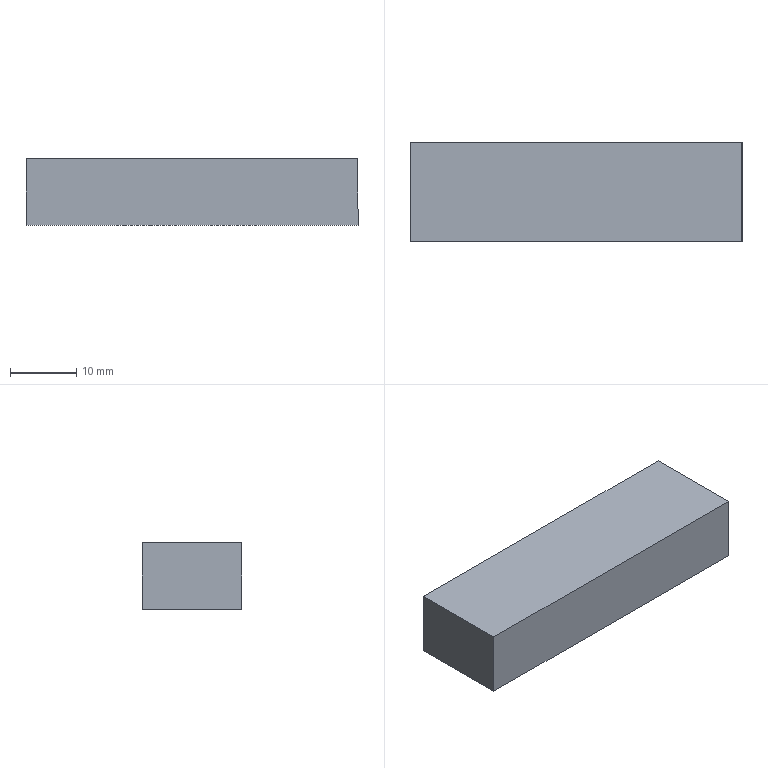Part | 4 solids | 50 faces | box 50 x 15 x 10 mm | volume 12752 mm3 | plane 42 | cylinder 8 | commonest cylinder face diameters 2.5 x4 3 x4
STEP:
#1=CARTESIAN_POINT('',(6.,12.,-2.5));
#2=VERTEX_POINT('',#1);
#3=CARTESIAN_POINT('',(6.,12.,7.5));
#4=VERTEX_POINT('',#3);
#5=CARTESIAN_POINT('',(6.,12.,2.5));
#6=DIRECTION('',(0.,0.,1.));
#7=VECTOR('',#6,1000.);
#8=LINE('',#5,#7);
#9=EDGE_CURVE('',#2,#4,#8,.T.);
#10=ORIENTED_EDGE('',*,*,#9,.F.);
#11=CARTESIAN_POINT('',(-44.,12.,-2.5));
#12=VERTEX_POINT('',#11);
#13=CARTESIAN_POINT('',(-19.,12.,-2.5));
#14=DIRECTION('',(1.,0.,0.));
#15=VECTOR('',#14,1000.);
#16=LINE('',#13,#15);
#17=EDGE_CURVE('',#12,#2,#16,.T.);
#18=ORIENTED_EDGE('',*,*,#17,.F.);
#19=CARTESIAN_POINT('',(-44.,12.,7.5));
#20=VERTEX_POINT('',#19);
#21=CARTESIAN_POINT('',(-44.,12.,2.5));
#22=DIRECTION('',(0.,0.,-1.));
#23=VECTOR('',#22,1000.);
#24=LINE('',#21,#23);
#25=EDGE_CURVE('',#20,#12,#24,.T.);
#26=ORIENTED_EDGE('',*,*,#25,.F.);
#27=CARTESIAN_POINT('',(-19.,12.,7.5));
#28=DIRECTION('',(-1.,0.,0.));
#29=VECTOR('',#28,1000.);
#30=LINE('',#27,#29);
#31=EDGE_CURVE('',#4,#20,#30,.T.);
#32=ORIENTED_EDGE('',*,*,#31,.F.);
#33=EDGE_LOOP('',(#10,#18,#26,#32));
#34=FACE_BOUND('',#33,.T.);
#35=CARTESIAN_POINT('',(-19.,12.,2.5));
#36=DIRECTION('',(0.,1.,0.));
#37=DIRECTION('',(0.,0.,1.));
#38=AXIS2_PLACEMENT_3D('',#35,#36,#37);
#39=PLANE('',#38);
#40=ADVANCED_FACE('',(#34),#39,.T.);
#41=CARTESIAN_POINT('',(6.,-3.,-2.5));
#42=VERTEX_POINT('',#41);
#43=CARTESIAN_POINT('',(6.,-3.,-2.5));
#44=DIRECTION('',(0.,1.,0.));
#45=VECTOR('',#44,1000.);
#46=LINE('',#43,#45);
#47=EDGE_CURVE('',#42,#2,#46,.T.);
#48=ORIENTED_EDGE('',*,*,#47,.T.);
#49=ORIENTED_EDGE('',*,*,#9,.T.);
#50=CARTESIAN_POINT('',(6.,-3.,7.5));
#51=VERTEX_POINT('',#50);
#52=CARTESIAN_POINT('',(6.,-3.,7.5));
#53=DIRECTION('',(0.,1.,0.));
#54=VECTOR('',#53,1000.);
#55=LINE('',#52,#54);
#56=EDGE_CURVE('',#51,#4,#55,.T.);
#57=ORIENTED_EDGE('',*,*,#56,.F.);
#58=CARTESIAN_POINT('',(6.,-3.,2.5));
#59=DIRECTION('',(0.,0.,-1.));
#60=VECTOR('',#59,1000.);
#61=LINE('',#58,#60);
#62=EDGE_CURVE('',#51,#42,#61,.T.);
#63=ORIENTED_EDGE('',*,*,#62,.T.);
#64=EDGE_LOOP('',(#48,#49,#57,#63));
#65=FACE_BOUND('',#64,.T.);
#66=CARTESIAN_POINT('',(6.,-3.,2.5));
#67=DIRECTION('',(1.,0.,0.));
#68=DIRECTION('',(0.,0.,-1.));
#69=AXIS2_PLACEMENT_3D('',#66,#67,#68);
#70=PLANE('',#69);
#71=ADVANCED_FACE('',(#65),#70,.T.);
#72=ORIENTED_EDGE('',*,*,#56,.T.);
#73=ORIENTED_EDGE('',*,*,#31,.T.);
#74=CARTESIAN_POINT('',(-44.,-3.,7.5));
#75=VERTEX_POINT('',#74);
#76=CARTESIAN_POINT('',(-44.,-3.,7.5));
#77=DIRECTION('',(0.,1.,0.));
#78=VECTOR('',#77,1000.);
#79=LINE('',#76,#78);
#80=EDGE_CURVE('',#75,#20,#79,.T.);
#81=ORIENTED_EDGE('',*,*,#80,.F.);
#82=CARTESIAN_POINT('',(-19.,-3.,7.5));
#83=DIRECTION('',(1.,0.,0.));
#84=VECTOR('',#83,1000.);
#85=LINE('',#82,#84);
#86=EDGE_CURVE('',#75,#51,#85,.T.);
#87=ORIENTED_EDGE('',*,*,#86,.T.);
#88=EDGE_LOOP('',(#72,#73,#81,#87));
#89=FACE_BOUND('',#88,.T.);
#90=CARTESIAN_POINT('',(-19.,-3.,7.5));
#91=DIRECTION('',(0.,0.,1.));
#92=DIRECTION('',(1.,0.,0.));
#93=AXIS2_PLACEMENT_3D('',#90,#91,#92);
#94=PLANE('',#93);
#95=ADVANCED_FACE('',(#89),#94,.T.);
#96=ORIENTED_EDGE('',*,*,#80,.T.);
#97=ORIENTED_EDGE('',*,*,#25,.T.);
#98=CARTESIAN_POINT('',(-44.,-3.,-2.5));
#99=VERTEX_POINT('',#98);
#100=CARTESIAN_POINT('',(-44.,-3.,-2.5));
#101=DIRECTION('',(0.,1.,0.));
#102=VECTOR('',#101,1000.);
#103=LINE('',#100,#102);
#104=EDGE_CURVE('',#99,#12,#103,.T.);
#105=ORIENTED_EDGE('',*,*,#104,.F.);
#106=CARTESIAN_POINT('',(-44.,-3.,2.5));
#107=DIRECTION('',(0.,0.,1.));
#108=VECTOR('',#107,1000.);
#109=LINE('',#106,#108);
#110=EDGE_CURVE('',#99,#75,#109,.T.);
#111=ORIENTED_EDGE('',*,*,#110,.T.);
#112=EDGE_LOOP('',(#96,#97,#105,#111));
#113=FACE_BOUND('',#112,.T.);
#114=CARTESIAN_POINT('',(-44.,-3.,2.5));
#115=DIRECTION('',(-1.,0.,0.));
#116=DIRECTION('',(0.,0.,1.));
#117=AXIS2_PLACEMENT_3D('',#114,#115,#116);
#118=PLANE('',#117);
#119=ADVANCED_FACE('',(#113),#118,.T.);
#120=CARTESIAN_POINT('',(-19.,-3.,-2.5));
#121=DIRECTION('',(-1.,0.,0.));
#122=VECTOR('',#121,1000.);
#123=LINE('',#120,#122);
#124=EDGE_CURVE('',#42,#99,#123,.T.);
#125=ORIENTED_EDGE('',*,*,#124,.F.);
#126=ORIENTED_EDGE('',*,*,#62,.F.);
#127=ORIENTED_EDGE('',*,*,#86,.F.);
#128=ORIENTED_EDGE('',*,*,#110,.F.);
#129=EDGE_LOOP('',(#125,#126,#127,#128));
#130=FACE_BOUND('',#129,.T.);
#131=CARTESIAN_POINT('',(-19.,-3.,2.5));
#132=DIRECTION('',(0.,-1.,0.));
#133=DIRECTION('',(0.,0.,-1.));
#134=AXIS2_PLACEMENT_3D('',#131,#132,#133);
#135=PLANE('',#134);
#136=ADVANCED_FACE('',(#130),#135,.T.);
#137=ORIENTED_EDGE('',*,*,#124,.T.);
#138=ORIENTED_EDGE('',*,*,#104,.T.);
#139=ORIENTED_EDGE('',*,*,#17,.T.);
#140=ORIENTED_EDGE('',*,*,#47,.F.);
#141=EDGE_LOOP('',(#137,#138,#139,#140));
#142=FACE_BOUND('',#141,.T.);
#143=CARTESIAN_POINT('',(-19.,-3.,-2.5));
#144=DIRECTION('',(0.,0.,-1.));
#145=DIRECTION('',(-1.,0.,0.));
#146=AXIS2_PLACEMENT_3D('',#143,#144,#145);
#147=PLANE('',#146);
#148=ADVANCED_FACE('',(#142),#147,.T.);
#149=CLOSED_SHELL('',(#40,#71,#95,#119,#136,#148));
#150=MANIFOLD_SOLID_BREP('',#149);
#151=CARTESIAN_POINT('',(0.,10.,0.));
#152=VERTEX_POINT('',#151);
#153=CARTESIAN_POINT('',(0.,10.,5.));
#154=VERTEX_POINT('',#153);
#155=CARTESIAN_POINT('',(0.,10.,2.5));
#156=DIRECTION('',(0.,0.,1.));
#157=VECTOR('',#156,1000.);
#158=LINE('',#155,#157);
#159=EDGE_CURVE('',#152,#154,#158,.T.);
#160=ORIENTED_EDGE('',*,*,#159,.F.);
#161=CARTESIAN_POINT('',(-41.,10.,0.));
#162=VERTEX_POINT('',#161);
#163=CARTESIAN_POINT('',(-20.5,10.,0.));
#164=DIRECTION('',(1.,0.,0.));
#165=VECTOR('',#164,1000.);
#166=LINE('',#163,#165);
#167=EDGE_CURVE('',#162,#152,#166,.T.);
#168=ORIENTED_EDGE('',*,*,#167,.F.);
#169=CARTESIAN_POINT('',(-41.,10.,5.));
#170=VERTEX_POINT('',#169);
#171=CARTESIAN_POINT('',(-41.,10.,2.5));
#172=DIRECTION('',(0.,0.,-1.));
#173=VECTOR('',#172,1000.);
#174=LINE('',#171,#173);
#175=EDGE_CURVE('',#170,#162,#174,.T.);
#176=ORIENTED_EDGE('',*,*,#175,.F.);
#177=CARTESIAN_POINT('',(-20.5,10.,5.));
#178=DIRECTION('',(-1.,0.,0.));
#179=VECTOR('',#178,1000.);
#180=LINE('',#177,#179);
#181=EDGE_CURVE('',#154,#170,#180,.T.);
#182=ORIENTED_EDGE('',*,*,#181,.F.);
#183=EDGE_LOOP('',(#160,#168,#176,#182));
#184=FACE_BOUND('',#183,.T.);
#185=CARTESIAN_POINT('',(-20.5,10.,2.5));
#186=DIRECTION('',(0.,1.,0.));
#187=DIRECTION('',(0.,0.,1.));
#188=AXIS2_PLACEMENT_3D('',#185,#186,#187);
#189=PLANE('',#188);
#190=ADVANCED_FACE('',(#184),#189,.T.);
#191=CARTESIAN_POINT('',(0.,0.,0.));
#192=VERTEX_POINT('',#191);
#193=CARTESIAN_POINT('',(0.,0.,0.));
#194=DIRECTION('',(0.,1.,0.));
#195=VECTOR('',#194,1000.);
#196=LINE('',#193,#195);
#197=EDGE_CURVE('',#192,#152,#196,.T.);
#198=ORIENTED_EDGE('',*,*,#197,.T.);
#199=ORIENTED_EDGE('',*,*,#159,.T.);
#200=CARTESIAN_POINT('',(0.,0.,5.));
#201=VERTEX_POINT('',#200);
#202=CARTESIAN_POINT('',(0.,0.,5.));
#203=DIRECTION('',(0.,1.,0.));
#204=VECTOR('',#203,1000.);
#205=LINE('',#202,#204);
#206=EDGE_CURVE('',#201,#154,#205,.T.);
#207=ORIENTED_EDGE('',*,*,#206,.F.);
#208=CARTESIAN_POINT('',(0.,0.,2.5));
#209=DIRECTION('',(0.,0.,-1.));
#210=VECTOR('',#209,1000.);
#211=LINE('',#208,#210);
#212=EDGE_CURVE('',#201,#192,#211,.T.);
#213=ORIENTED_EDGE('',*,*,#212,.T.);
#214=EDGE_LOOP('',(#198,#199,#207,#213));
#215=FACE_BOUND('',#214,.T.);
#216=CARTESIAN_POINT('',(0.,0.,2.5));
#217=DIRECTION('',(1.,0.,0.));
#218=DIRECTION('',(0.,0.,-1.));
#219=AXIS2_PLACEMENT_3D('',#216,#217,#218);
#220=PLANE('',#219);
#221=ADVANCED_FACE('',(#215),#220,.T.);
#222=ORIENTED_EDGE('',*,*,#206,.T.);
#223=ORIENTED_EDGE('',*,*,#181,.T.);
#224=CARTESIAN_POINT('',(-41.,0.,5.));
#225=VERTEX_POINT('',#224);
#226=CARTESIAN_POINT('',(-41.,0.,5.));
#227=DIRECTION('',(0.,1.,0.));
#228=VECTOR('',#227,1000.);
#229=LINE('',#226,#228);
#230=EDGE_CURVE('',#225,#170,#229,.T.);
#231=ORIENTED_EDGE('',*,*,#230,.F.);
#232=CARTESIAN_POINT('',(-20.5,0.,5.));
#233=DIRECTION('',(1.,0.,0.));
#234=VECTOR('',#233,1000.);
#235=LINE('',#232,#234);
#236=EDGE_CURVE('',#225,#201,#235,.T.);
#237=ORIENTED_EDGE('',*,*,#236,.T.);
#238=EDGE_LOOP('',(#222,#223,#231,#237));
#239=FACE_BOUND('',#238,.T.);
#240=CARTESIAN_POINT('',(-20.5,0.,5.));
#241=DIRECTION('',(0.,0.,1.));
#242=DIRECTION('',(1.,0.,0.));
#243=AXIS2_PLACEMENT_3D('',#240,#241,#242);
#244=PLANE('',#243);
#245=ADVANCED_FACE('',(#239),#244,.T.);
#246=ORIENTED_EDGE('',*,*,#230,.T.);
#247=ORIENTED_EDGE('',*,*,#175,.T.);
#248=CARTESIAN_POINT('',(-41.,0.,0.));
#249=VERTEX_POINT('',#248);
#250=CARTESIAN_POINT('',(-41.,0.,0.));
#251=DIRECTION('',(0.,1.,0.));
#252=VECTOR('',#251,1000.);
#253=LINE('',#250,#252);
#254=EDGE_CURVE('',#249,#162,#253,.T.);
#255=ORIENTED_EDGE('',*,*,#254,.F.);
#256=CARTESIAN_POINT('',(-41.,0.,2.5));
#257=DIRECTION('',(0.,0.,1.));
#258=VECTOR('',#257,1000.);
#259=LINE('',#256,#258);
#260=EDGE_CURVE('',#249,#225,#259,.T.);
#261=ORIENTED_EDGE('',*,*,#260,.T.);
#262=EDGE_LOOP('',(#246,#247,#255,#261));
#263=FACE_BOUND('',#262,.T.);
#264=CARTESIAN_POINT('',(-41.,0.,2.5));
#265=DIRECTION('',(-1.,0.,0.));
#266=DIRECTION('',(0.,0.,1.));
#267=AXIS2_PLACEMENT_3D('',#264,#265,#266);
#268=PLANE('',#267);
#269=ADVANCED_FACE('',(#263),#268,.T.);
#270=CARTESIAN_POINT('',(-20.5,0.,0.));
#271=DIRECTION('',(-1.,0.,0.));
#272=VECTOR('',#271,1000.);
#273=LINE('',#270,#272);
#274=EDGE_CURVE('',#192,#249,#273,.T.);
#275=ORIENTED_EDGE('',*,*,#274,.F.);
#276=ORIENTED_EDGE('',*,*,#212,.F.);
#277=ORIENTED_EDGE('',*,*,#236,.F.);
#278=ORIENTED_EDGE('',*,*,#260,.F.);
#279=EDGE_LOOP('',(#275,#276,#277,#278));
#280=FACE_BOUND('',#279,.T.);
#281=CARTESIAN_POINT('',(-20.5,0.,2.5));
#282=DIRECTION('',(0.,-1.,0.));
#283=DIRECTION('',(0.,0.,-1.));
#284=AXIS2_PLACEMENT_3D('',#281,#282,#283);
#285=PLANE('',#284);
#286=ADVANCED_FACE('',(#280),#285,.T.);
#287=ORIENTED_EDGE('',*,*,#274,.T.);
#288=ORIENTED_EDGE('',*,*,#254,.T.);
#289=ORIENTED_EDGE('',*,*,#167,.T.);
#290=ORIENTED_EDGE('',*,*,#197,.F.);
#291=EDGE_LOOP('',(#287,#288,#289,#290));
#292=FACE_BOUND('',#291,.T.);
#293=CARTESIAN_POINT('',(-20.5,0.,0.));
#294=DIRECTION('',(0.,0.,-1.));
#295=DIRECTION('',(-1.,0.,0.));
#296=AXIS2_PLACEMENT_3D('',#293,#294,#295);
#297=PLANE('',#296);
#298=ADVANCED_FACE('',(#292),#297,.T.);
#299=CLOSED_SHELL('',(#190,#221,#245,#269,#286,#298));
#300=MANIFOLD_SOLID_BREP('',#299);
#301=CARTESIAN_POINT('',(-6.,2.5,4.));
#302=VERTEX_POINT('',#301);
#303=CARTESIAN_POINT('',(-6.,2.5,1.));
#304=VERTEX_POINT('',#303);
#305=CARTESIAN_POINT('',(-6.,2.5,2.5));
#306=DIRECTION('',(1.,0.,0.));
#307=DIRECTION('',(0.,0.,-1.));
#308=AXIS2_PLACEMENT_3D('',#305,#306,#307);
#309=CIRCLE('',#308,1.5);
#310=EDGE_CURVE('',#302,#304,#309,.T.);
#311=ORIENTED_EDGE('',*,*,#310,.F.);
#312=CARTESIAN_POINT('',(0.,2.5,4.));
#313=VERTEX_POINT('',#312);
#314=CARTESIAN_POINT('',(-6.,2.5,4.));
#315=DIRECTION('',(1.,0.,0.));
#316=VECTOR('',#315,1000.);
#317=LINE('',#314,#316);
#318=EDGE_CURVE('',#302,#313,#317,.T.);
#319=ORIENTED_EDGE('',*,*,#318,.T.);
#320=CARTESIAN_POINT('',(0.,2.5,1.));
#321=VERTEX_POINT('',#320);
#322=CARTESIAN_POINT('',(0.,2.5,2.5));
#323=DIRECTION('',(1.,0.,0.));
#324=DIRECTION('',(0.,0.,-1.));
#325=AXIS2_PLACEMENT_3D('',#322,#323,#324);
#326=CIRCLE('',#325,1.5);
#327=EDGE_CURVE('',#313,#321,#326,.T.);
#328=ORIENTED_EDGE('',*,*,#327,.T.);
#329=CARTESIAN_POINT('',(-6.,2.5,1.));
#330=DIRECTION('',(1.,0.,0.));
#331=VECTOR('',#330,1000.);
#332=LINE('',#329,#331);
#333=EDGE_CURVE('',#304,#321,#332,.T.);
#334=ORIENTED_EDGE('',*,*,#333,.F.);
#335=EDGE_LOOP('',(#311,#319,#328,#334));
#336=FACE_BOUND('',#335,.T.);
#337=CARTESIAN_POINT('',(-6.,2.5,2.5));
#338=DIRECTION('',(1.,0.,0.));
#339=DIRECTION('',(0.,0.,1.));
#340=AXIS2_PLACEMENT_3D('',#337,#338,#339);
#341=CYLINDRICAL_SURFACE('',#340,1.5);
#342=ADVANCED_FACE('',(#336),#341,.F.);
#343=CARTESIAN_POINT('',(-1.85,5.,2.5));
#344=VERTEX_POINT('',#343);
#345=CARTESIAN_POINT('',(-4.35,5.,2.5));
#346=VERTEX_POINT('',#345);
#347=CARTESIAN_POINT('',(-3.1,5.,2.5));
#348=DIRECTION('',(0.,1.,0.));
#349=DIRECTION('',(-1.,0.,0.));
#350=AXIS2_PLACEMENT_3D('',#347,#348,#349);
#351=CIRCLE('',#350,1.25);
#352=EDGE_CURVE('',#344,#346,#351,.T.);
#353=ORIENTED_EDGE('',*,*,#352,.F.);
#354=CARTESIAN_POINT('',(-1.85,10.,2.5));
#355=VERTEX_POINT('',#354);
#356=CARTESIAN_POINT('',(-1.85,5.,2.5));
#357=DIRECTION('',(0.,1.,0.));
#358=VECTOR('',#357,1000.);
#359=LINE('',#356,#358);
#360=EDGE_CURVE('',#344,#355,#359,.T.);
#361=ORIENTED_EDGE('',*,*,#360,.T.);
#362=CARTESIAN_POINT('',(-4.35,10.,2.5));
#363=VERTEX_POINT('',#362);
#364=CARTESIAN_POINT('',(-3.1,10.,2.5));
#365=DIRECTION('',(0.,1.,0.));
#366=DIRECTION('',(-1.,0.,0.));
#367=AXIS2_PLACEMENT_3D('',#364,#365,#366);
#368=CIRCLE('',#367,1.25);
#369=EDGE_CURVE('',#355,#363,#368,.T.);
#370=ORIENTED_EDGE('',*,*,#369,.T.);
#371=CARTESIAN_POINT('',(-4.35,5.,2.5));
#372=DIRECTION('',(0.,1.,0.));
#373=VECTOR('',#372,1000.);
#374=LINE('',#371,#373);
#375=EDGE_CURVE('',#346,#363,#374,.T.);
#376=ORIENTED_EDGE('',*,*,#375,.F.);
#377=EDGE_LOOP('',(#353,#361,#370,#376));
#378=FACE_BOUND('',#377,.T.);
#379=CARTESIAN_POINT('',(-3.1,5.,2.5));
#380=DIRECTION('',(0.,1.,0.));
#381=DIRECTION('',(1.,0.,0.));
#382=AXIS2_PLACEMENT_3D('',#379,#380,#381);
#383=CYLINDRICAL_SURFACE('',#382,1.25);
#384=ADVANCED_FACE('',(#378),#383,.F.);
#385=CARTESIAN_POINT('',(-36.65,5.,2.5));
#386=VERTEX_POINT('',#385);
#387=CARTESIAN_POINT('',(-39.15,5.,2.5));
#388=VERTEX_POINT('',#387);
#389=CARTESIAN_POINT('',(-37.9,5.,2.5));
#390=DIRECTION('',(0.,1.,0.));
#391=DIRECTION('',(-1.,0.,0.));
#392=AXIS2_PLACEMENT_3D('',#389,#390,#391);
#393=CIRCLE('',#392,1.25);
#394=EDGE_CURVE('',#386,#388,#393,.T.);
#395=ORIENTED_EDGE('',*,*,#394,.F.);
#396=CARTESIAN_POINT('',(-36.65,10.,2.5));
#397=VERTEX_POINT('',#396);
#398=CARTESIAN_POINT('',(-36.65,5.,2.5));
#399=DIRECTION('',(0.,1.,0.));
#400=VECTOR('',#399,1000.);
#401=LINE('',#398,#400);
#402=EDGE_CURVE('',#386,#397,#401,.T.);
#403=ORIENTED_EDGE('',*,*,#402,.T.);
#404=CARTESIAN_POINT('',(-39.15,10.,2.5));
#405=VERTEX_POINT('',#404);
#406=CARTESIAN_POINT('',(-37.9,10.,2.5));
#407=DIRECTION('',(0.,1.,0.));
#408=DIRECTION('',(-1.,0.,0.));
#409=AXIS2_PLACEMENT_3D('',#406,#407,#408);
#410=CIRCLE('',#409,1.25);
#411=EDGE_CURVE('',#397,#405,#410,.T.);
#412=ORIENTED_EDGE('',*,*,#411,.T.);
#413=CARTESIAN_POINT('',(-39.15,5.,2.5));
#414=DIRECTION('',(0.,1.,0.));
#415=VECTOR('',#414,1000.);
#416=LINE('',#413,#415);
#417=EDGE_CURVE('',#388,#405,#416,.T.);
#418=ORIENTED_EDGE('',*,*,#417,.F.);
#419=EDGE_LOOP('',(#395,#403,#412,#418));
#420=FACE_BOUND('',#419,.T.);
#421=CARTESIAN_POINT('',(-37.9,5.,2.5));
#422=DIRECTION('',(0.,1.,0.));
#423=DIRECTION('',(1.,0.,0.));
#424=AXIS2_PLACEMENT_3D('',#421,#422,#423);
#425=CYLINDRICAL_SURFACE('',#424,1.25);
#426=ADVANCED_FACE('',(#420),#425,.F.);
#427=CARTESIAN_POINT('',(0.,2.5,2.5));
#428=DIRECTION('',(1.,0.,0.));
#429=DIRECTION('',(0.,0.,-1.));
#430=AXIS2_PLACEMENT_3D('',#427,#428,#429);
#431=CIRCLE('',#430,1.5);
#432=EDGE_CURVE('',#321,#313,#431,.T.);
#433=ORIENTED_EDGE('',*,*,#432,.F.);
#434=ORIENTED_EDGE('',*,*,#327,.F.);
#435=EDGE_LOOP('',(#433,#434));
#436=FACE_BOUND('',#435,.T.);
#437=CARTESIAN_POINT('',(0.,0.,4.9));
#438=VERTEX_POINT('',#437);
#439=CARTESIAN_POINT('',(0.,0.,0.1));
#440=VERTEX_POINT('',#439);
#441=CARTESIAN_POINT('',(0.,0.,5.));
#442=DIRECTION('',(0.,0.,-1.));
#443=VECTOR('',#442,1000.);
#444=LINE('',#441,#443);
#445=EDGE_CURVE('',#438,#440,#444,.T.);
#446=ORIENTED_EDGE('',*,*,#445,.T.);
#447=CARTESIAN_POINT('',(0.,10.,0.1));
#448=VERTEX_POINT('',#447);
#449=CARTESIAN_POINT('',(0.,0.,0.1));
#450=DIRECTION('',(0.,1.,0.));
#451=VECTOR('',#450,1000.);
#452=LINE('',#449,#451);
#453=EDGE_CURVE('',#440,#448,#452,.T.);
#454=ORIENTED_EDGE('',*,*,#453,.T.);
#455=CARTESIAN_POINT('',(0.,10.,4.9));
#456=VERTEX_POINT('',#455);
#457=CARTESIAN_POINT('',(0.,10.,5.));
#458=DIRECTION('',(0.,0.,-1.));
#459=VECTOR('',#458,1000.);
#460=LINE('',#457,#459);
#461=EDGE_CURVE('',#456,#448,#460,.T.);
#462=ORIENTED_EDGE('',*,*,#461,.F.);
#463=CARTESIAN_POINT('',(0.,0.,4.9));
#464=DIRECTION('',(0.,-1.,0.));
#465=VECTOR('',#464,1000.);
#466=LINE('',#463,#465);
#467=EDGE_CURVE('',#456,#438,#466,.T.);
#468=ORIENTED_EDGE('',*,*,#467,.T.);
#469=EDGE_LOOP('',(#446,#454,#462,#468));
#470=FACE_BOUND('',#469,.T.);
#471=CARTESIAN_POINT('',(0.,0.,5.));
#472=DIRECTION('',(-1.,0.,0.));
#473=DIRECTION('',(0.,0.,-1.));
#474=AXIS2_PLACEMENT_3D('',#471,#472,#473);
#475=PLANE('',#474);
#476=ADVANCED_FACE('',(#436,#470),#475,.F.);
#477=CARTESIAN_POINT('',(-3.1,10.,2.5));
#478=DIRECTION('',(0.,1.,0.));
#479=DIRECTION('',(-1.,0.,0.));
#480=AXIS2_PLACEMENT_3D('',#477,#478,#479);
#481=CIRCLE('',#480,1.25);
#482=EDGE_CURVE('',#363,#355,#481,.T.);
#483=ORIENTED_EDGE('',*,*,#482,.F.);
#484=ORIENTED_EDGE('',*,*,#369,.F.);
#485=EDGE_LOOP('',(#483,#484));
#486=FACE_BOUND('',#485,.T.);
#487=ORIENTED_EDGE('',*,*,#461,.T.);
#488=CARTESIAN_POINT('',(-0.1,10.,0.));
#489=VERTEX_POINT('',#488);
#490=CARTESIAN_POINT('',(0.,10.,0.1));
#491=DIRECTION('',(0.7071,0.,0.7071));
#492=VECTOR('',#491,1000.);
#493=LINE('',#490,#492);
#494=EDGE_CURVE('',#448,#489,#493,.F.);
#495=ORIENTED_EDGE('',*,*,#494,.T.);
#496=CARTESIAN_POINT('',(-4.6,10.,0.));
#497=VERTEX_POINT('',#496);
#498=CARTESIAN_POINT('',(0.,10.,0.));
#499=DIRECTION('',(-1.,0.,0.));
#500=VECTOR('',#499,1000.);
#501=LINE('',#498,#500);
#502=EDGE_CURVE('',#489,#497,#501,.T.);
#503=ORIENTED_EDGE('',*,*,#502,.T.);
#504=CARTESIAN_POINT('',(-4.6,10.,5.));
#505=VERTEX_POINT('',#504);
#506=CARTESIAN_POINT('',(-4.6,10.,5.));
#507=DIRECTION('',(0.,0.,1.));
#508=VECTOR('',#507,1000.);
#509=LINE('',#506,#508);
#510=EDGE_CURVE('',#497,#505,#509,.T.);
#511=ORIENTED_EDGE('',*,*,#510,.T.);
#512=CARTESIAN_POINT('',(-0.1,10.,5.));
#513=VERTEX_POINT('',#512);
#514=CARTESIAN_POINT('',(0.,10.,5.));
#515=DIRECTION('',(-1.,0.,0.));
#516=VECTOR('',#515,1000.);
#517=LINE('',#514,#516);
#518=EDGE_CURVE('',#513,#505,#517,.T.);
#519=ORIENTED_EDGE('',*,*,#518,.F.);
#520=CARTESIAN_POINT('',(-0.1,10.,5.));
#521=DIRECTION('',(0.7071,0.,-0.7071));
#522=VECTOR('',#521,1000.);
#523=LINE('',#520,#522);
#524=EDGE_CURVE('',#513,#456,#523,.T.);
#525=ORIENTED_EDGE('',*,*,#524,.T.);
#526=EDGE_LOOP('',(#487,#495,#503,#511,#519,#525));
#527=FACE_BOUND('',#526,.T.);
#528=CARTESIAN_POINT('',(0.,10.,5.));
#529=DIRECTION('',(0.,-1.,0.));
#530=DIRECTION('',(-1.,0.,0.));
#531=AXIS2_PLACEMENT_3D('',#528,#529,#530);
#532=PLANE('',#531);
#533=ADVANCED_FACE('',(#486,#527),#532,.F.);
#534=CARTESIAN_POINT('',(-5.1,9.5,5.));
#535=VERTEX_POINT('',#534);
#536=CARTESIAN_POINT('',(-5.1,6.5,5.));
#537=VERTEX_POINT('',#536);
#538=CARTESIAN_POINT('',(-5.1,10.,5.));
#539=DIRECTION('',(0.,-1.,0.));
#540=VECTOR('',#539,1000.);
#541=LINE('',#538,#540);
#542=EDGE_CURVE('',#535,#537,#541,.T.);
#543=ORIENTED_EDGE('',*,*,#542,.F.);
#544=CARTESIAN_POINT('',(-5.1,9.5,0.));
#545=VERTEX_POINT('',#544);
#546=CARTESIAN_POINT('',(-5.1,9.5,5.));
#547=DIRECTION('',(0.,0.,-1.));
#548=VECTOR('',#547,1000.);
#549=LINE('',#546,#548);
#550=EDGE_CURVE('',#535,#545,#549,.T.);
#551=ORIENTED_EDGE('',*,*,#550,.T.);
#552=CARTESIAN_POINT('',(-5.1,6.5,0.));
#553=VERTEX_POINT('',#552);
#554=CARTESIAN_POINT('',(-5.1,10.,0.));
#555=DIRECTION('',(0.,-1.,0.));
#556=VECTOR('',#555,1000.);
#557=LINE('',#554,#556);
#558=EDGE_CURVE('',#545,#553,#557,.T.);
#559=ORIENTED_EDGE('',*,*,#558,.T.);
#560=CARTESIAN_POINT('',(-5.1,6.5,5.));
#561=DIRECTION('',(0.,0.,1.));
#562=VECTOR('',#561,1000.);
#563=LINE('',#560,#562);
#564=EDGE_CURVE('',#553,#537,#563,.T.);
#565=ORIENTED_EDGE('',*,*,#564,.T.);
#566=EDGE_LOOP('',(#543,#551,#559,#565));
#567=FACE_BOUND('',#566,.T.);
#568=CARTESIAN_POINT('',(-5.1,10.,5.));
#569=DIRECTION('',(1.,0.,0.));
#570=DIRECTION('',(0.,0.,1.));
#571=AXIS2_PLACEMENT_3D('',#568,#569,#570);
#572=PLANE('',#571);
#573=ADVANCED_FACE('',(#567),#572,.F.);
#574=CARTESIAN_POINT('',(-6.6,5.,5.));
#575=VERTEX_POINT('',#574);
#576=CARTESIAN_POINT('',(-34.4,5.,5.));
#577=VERTEX_POINT('',#576);
#578=CARTESIAN_POINT('',(-35.9,5.,5.));
#579=DIRECTION('',(-1.,0.,0.));
#580=VECTOR('',#579,1000.);
#581=LINE('',#578,#580);
#582=EDGE_CURVE('',#575,#577,#581,.T.);
#583=ORIENTED_EDGE('',*,*,#582,.F.);
#584=CARTESIAN_POINT('',(-6.6,5.,0.));
#585=VERTEX_POINT('',#584);
#586=CARTESIAN_POINT('',(-6.6,5.,0.));
#587=DIRECTION('',(0.,0.,-1.));
#588=VECTOR('',#587,1000.);
#589=LINE('',#586,#588);
#590=EDGE_CURVE('',#575,#585,#589,.T.);
#591=ORIENTED_EDGE('',*,*,#590,.T.);
#592=CARTESIAN_POINT('',(-34.4,5.,0.));
#593=VERTEX_POINT('',#592);
#594=CARTESIAN_POINT('',(-35.9,5.,0.));
#595=DIRECTION('',(-1.,0.,0.));
#596=VECTOR('',#595,1000.);
#597=LINE('',#594,#596);
#598=EDGE_CURVE('',#585,#593,#597,.T.);
#599=ORIENTED_EDGE('',*,*,#598,.T.);
#600=CARTESIAN_POINT('',(-34.4,5.,5.));
#601=DIRECTION('',(0.,0.,1.));
#602=VECTOR('',#601,1000.);
#603=LINE('',#600,#602);
#604=EDGE_CURVE('',#593,#577,#603,.T.);
#605=ORIENTED_EDGE('',*,*,#604,.T.);
#606=EDGE_LOOP('',(#583,#591,#599,#605));
#607=FACE_BOUND('',#606,.T.);
#608=CARTESIAN_POINT('',(-35.9,5.,5.));
#609=DIRECTION('',(0.,-1.,0.));
#610=DIRECTION('',(0.,0.,1.));
#611=AXIS2_PLACEMENT_3D('',#608,#609,#610);
#612=PLANE('',#611);
#613=ADVANCED_FACE('',(#607),#612,.F.);
#614=CARTESIAN_POINT('',(-35.9,6.5,0.));
#615=VERTEX_POINT('',#614);
#616=CARTESIAN_POINT('',(-35.9,9.5,0.));
#617=VERTEX_POINT('',#616);
#618=CARTESIAN_POINT('',(-35.9,10.,0.));
#619=DIRECTION('',(0.,1.,0.));
#620=VECTOR('',#619,1000.);
#621=LINE('',#618,#620);
#622=EDGE_CURVE('',#615,#617,#621,.T.);
#623=ORIENTED_EDGE('',*,*,#622,.T.);
#624=CARTESIAN_POINT('',(-35.9,9.5,5.));
#625=VERTEX_POINT('',#624);
#626=CARTESIAN_POINT('',(-35.9,9.5,5.));
#627=DIRECTION('',(0.,0.,1.));
#628=VECTOR('',#627,1000.);
#629=LINE('',#626,#628);
#630=EDGE_CURVE('',#617,#625,#629,.T.);
#631=ORIENTED_EDGE('',*,*,#630,.T.);
#632=CARTESIAN_POINT('',(-35.9,6.5,5.));
#633=VERTEX_POINT('',#632);
#634=CARTESIAN_POINT('',(-35.9,10.,5.));
#635=DIRECTION('',(0.,1.,0.));
#636=VECTOR('',#635,1000.);
#637=LINE('',#634,#636);
#638=EDGE_CURVE('',#633,#625,#637,.T.);
#639=ORIENTED_EDGE('',*,*,#638,.F.);
#640=CARTESIAN_POINT('',(-35.9,6.5,0.));
#641=DIRECTION('',(0.,0.,-1.));
#642=VECTOR('',#641,1000.);
#643=LINE('',#640,#642);
#644=EDGE_CURVE('',#633,#615,#643,.T.);
#645=ORIENTED_EDGE('',*,*,#644,.T.);
#646=EDGE_LOOP('',(#623,#631,#639,#645));
#647=FACE_BOUND('',#646,.T.);
#648=CARTESIAN_POINT('',(-35.9,10.,5.));
#649=DIRECTION('',(-1.,0.,0.));
#650=DIRECTION('',(0.,0.,-1.));
#651=AXIS2_PLACEMENT_3D('',#648,#649,#650);
#652=PLANE('',#651);
#653=ADVANCED_FACE('',(#647),#652,.F.);
#654=CARTESIAN_POINT('',(-37.9,10.,2.5));
#655=DIRECTION('',(0.,1.,0.));
#656=DIRECTION('',(-1.,0.,0.));
#657=AXIS2_PLACEMENT_3D('',#654,#655,#656);
#658=CIRCLE('',#657,1.25);
#659=EDGE_CURVE('',#405,#397,#658,.T.);
#660=ORIENTED_EDGE('',*,*,#659,.F.);
#661=ORIENTED_EDGE('',*,*,#411,.F.);
#662=EDGE_LOOP('',(#660,#661));
#663=FACE_BOUND('',#662,.T.);
#664=CARTESIAN_POINT('',(-36.4,10.,0.));
#665=VERTEX_POINT('',#664);
#666=CARTESIAN_POINT('',(-40.9,10.,0.));
#667=VERTEX_POINT('',#666);
#668=CARTESIAN_POINT('',(-35.9,10.,0.));
#669=DIRECTION('',(-1.,0.,0.));
#670=VECTOR('',#669,1000.);
#671=LINE('',#668,#670);
#672=EDGE_CURVE('',#665,#667,#671,.T.);
#673=ORIENTED_EDGE('',*,*,#672,.T.);
#674=CARTESIAN_POINT('',(-41.,10.,0.1));
#675=VERTEX_POINT('',#674);
#676=CARTESIAN_POINT('',(-41.,10.,0.1));
#677=DIRECTION('',(0.7071,0.,-0.7071));
#678=VECTOR('',#677,1000.);
#679=LINE('',#676,#678);
#680=EDGE_CURVE('',#667,#675,#679,.F.);
#681=ORIENTED_EDGE('',*,*,#680,.T.);
#682=CARTESIAN_POINT('',(-41.,10.,4.9));
#683=VERTEX_POINT('',#682);
#684=CARTESIAN_POINT('',(-41.,10.,5.));
#685=DIRECTION('',(0.,0.,-1.));
#686=VECTOR('',#685,1000.);
#687=LINE('',#684,#686);
#688=EDGE_CURVE('',#683,#675,#687,.T.);
#689=ORIENTED_EDGE('',*,*,#688,.F.);
#690=CARTESIAN_POINT('',(-40.9,10.,5.));
#691=VERTEX_POINT('',#690);
#692=CARTESIAN_POINT('',(-40.9,10.,5.));
#693=DIRECTION('',(0.7071,0.,0.7071));
#694=VECTOR('',#693,1000.);
#695=LINE('',#692,#694);
#696=EDGE_CURVE('',#683,#691,#695,.T.);
#697=ORIENTED_EDGE('',*,*,#696,.T.);
#698=CARTESIAN_POINT('',(-36.4,10.,5.));
#699=VERTEX_POINT('',#698);
#700=CARTESIAN_POINT('',(-35.9,10.,5.));
#701=DIRECTION('',(-1.,0.,0.));
#702=VECTOR('',#701,1000.);
#703=LINE('',#700,#702);
#704=EDGE_CURVE('',#699,#691,#703,.T.);
#705=ORIENTED_EDGE('',*,*,#704,.F.);
#706=CARTESIAN_POINT('',(-36.4,10.,5.));
#707=DIRECTION('',(0.,0.,-1.));
#708=VECTOR('',#707,1000.);
#709=LINE('',#706,#708);
#710=EDGE_CURVE('',#699,#665,#709,.T.);
#711=ORIENTED_EDGE('',*,*,#710,.T.);
#712=EDGE_LOOP('',(#673,#681,#689,#697,#705,#711));
#713=FACE_BOUND('',#712,.T.);
#714=CARTESIAN_POINT('',(-35.9,10.,5.));
#715=DIRECTION('',(0.,-1.,0.));
#716=DIRECTION('',(-1.,0.,0.));
#717=AXIS2_PLACEMENT_3D('',#714,#715,#716);
#718=PLANE('',#717);
#719=ADVANCED_FACE('',(#663,#713),#718,.F.);
#720=ORIENTED_EDGE('',*,*,#688,.T.);
#721=CARTESIAN_POINT('',(-41.,4.,0.1));
#722=VERTEX_POINT('',#721);
#723=CARTESIAN_POINT('',(-41.,0.,0.1));
#724=DIRECTION('',(0.,-1.,0.));
#725=VECTOR('',#724,1000.);
#726=LINE('',#723,#725);
#727=EDGE_CURVE('',#675,#722,#726,.T.);
#728=ORIENTED_EDGE('',*,*,#727,.T.);
#729=CARTESIAN_POINT('',(-41.,4.,4.9));
#730=VERTEX_POINT('',#729);
#731=CARTESIAN_POINT('',(-41.,4.,5.));
#732=DIRECTION('',(0.,0.,1.));
#733=VECTOR('',#732,1000.);
#734=LINE('',#731,#733);
#735=EDGE_CURVE('',#722,#730,#734,.T.);
#736=ORIENTED_EDGE('',*,*,#735,.T.);
#737=CARTESIAN_POINT('',(-41.,10.,4.9));
#738=DIRECTION('',(0.,1.,0.));
#739=VECTOR('',#738,1000.);
#740=LINE('',#737,#739);
#741=EDGE_CURVE('',#730,#683,#740,.T.);
#742=ORIENTED_EDGE('',*,*,#741,.T.);
#743=EDGE_LOOP('',(#720,#728,#736,#742));
#744=FACE_BOUND('',#743,.T.);
#745=CARTESIAN_POINT('',(-41.,0.,5.));
#746=DIRECTION('',(1.,0.,0.));
#747=DIRECTION('',(0.,0.,1.));
#748=AXIS2_PLACEMENT_3D('',#745,#746,#747);
#749=PLANE('',#748);
#750=ADVANCED_FACE('',(#744),#749,.F.);
#751=CARTESIAN_POINT('',(-37.,0.,0.));
#752=VERTEX_POINT('',#751);
#753=CARTESIAN_POINT('',(-0.1,0.,0.));
#754=VERTEX_POINT('',#753);
#755=CARTESIAN_POINT('',(0.,0.,0.));
#756=DIRECTION('',(1.,0.,0.));
#757=VECTOR('',#756,1000.);
#758=LINE('',#755,#757);
#759=EDGE_CURVE('',#752,#754,#758,.T.);
#760=ORIENTED_EDGE('',*,*,#759,.T.);
#761=CARTESIAN_POINT('',(0.,0.,0.1));
#762=DIRECTION('',(-0.7071,0.,-0.7071));
#763=VECTOR('',#762,1000.);
#764=LINE('',#761,#763);
#765=EDGE_CURVE('',#754,#440,#764,.F.);
#766=ORIENTED_EDGE('',*,*,#765,.T.);
#767=ORIENTED_EDGE('',*,*,#445,.F.);
#768=CARTESIAN_POINT('',(-0.1,0.,5.));
#769=VERTEX_POINT('',#768);
#770=CARTESIAN_POINT('',(-0.1,0.,5.));
#771=DIRECTION('',(-0.7071,0.,0.7071));
#772=VECTOR('',#771,1000.);
#773=LINE('',#770,#772);
#774=EDGE_CURVE('',#438,#769,#773,.T.);
#775=ORIENTED_EDGE('',*,*,#774,.T.);
#776=CARTESIAN_POINT('',(-37.,0.,5.));
#777=VERTEX_POINT('',#776);
#778=CARTESIAN_POINT('',(0.,0.,5.));
#779=DIRECTION('',(1.,0.,0.));
#780=VECTOR('',#779,1000.);
#781=LINE('',#778,#780);
#782=EDGE_CURVE('',#777,#769,#781,.T.);
#783=ORIENTED_EDGE('',*,*,#782,.F.);
#784=CARTESIAN_POINT('',(-37.,0.,5.));
#785=DIRECTION('',(0.,0.,-1.));
#786=VECTOR('',#785,1000.);
#787=LINE('',#784,#786);
#788=EDGE_CURVE('',#777,#752,#787,.T.);
#789=ORIENTED_EDGE('',*,*,#788,.T.);
#790=EDGE_LOOP('',(#760,#766,#767,#775,#783,#789));
#791=FACE_BOUND('',#790,.T.);
#792=CARTESIAN_POINT('',(0.,0.,5.));
#793=DIRECTION('',(0.,1.,0.));
#794=DIRECTION('',(0.,0.,-1.));
#795=AXIS2_PLACEMENT_3D('',#792,#793,#794);
#796=PLANE('',#795);
#797=ADVANCED_FACE('',(#791),#796,.F.);
#798=ORIENTED_EDGE('',*,*,#704,.T.);
#799=CARTESIAN_POINT('',(-40.9,3.9,5.));
#800=VERTEX_POINT('',#799);
#801=CARTESIAN_POINT('',(-40.9,4.,5.));
#802=DIRECTION('',(0.,-1.,0.));
#803=VECTOR('',#802,1000.);
#804=LINE('',#801,#803);
#805=EDGE_CURVE('',#691,#800,#804,.T.);
#806=ORIENTED_EDGE('',*,*,#805,.T.);
#807=CARTESIAN_POINT('',(-18.5,-18.5,5.));
#808=DIRECTION('',(0.7071,-0.7071,0.));
#809=VECTOR('',#808,1000.);
#810=LINE('',#807,#809);
#811=EDGE_CURVE('',#800,#777,#810,.T.);
#812=ORIENTED_EDGE('',*,*,#811,.T.);
#813=ORIENTED_EDGE('',*,*,#782,.T.);
#814=CARTESIAN_POINT('',(-0.1,10.,5.));
#815=DIRECTION('',(0.,1.,0.));
#816=VECTOR('',#815,1000.);
#817=LINE('',#814,#816);
#818=EDGE_CURVE('',#769,#513,#817,.T.);
#819=ORIENTED_EDGE('',*,*,#818,.T.);
#820=ORIENTED_EDGE('',*,*,#518,.T.);
#821=CARTESIAN_POINT('',(-7.3,7.3,5.));
#822=DIRECTION('',(-0.7071,-0.7071,0.));
#823=VECTOR('',#822,1000.);
#824=LINE('',#821,#823);
#825=EDGE_CURVE('',#505,#535,#824,.T.);
#826=ORIENTED_EDGE('',*,*,#825,.T.);
#827=ORIENTED_EDGE('',*,*,#542,.T.);
#828=CARTESIAN_POINT('',(-6.6,6.5,5.));
#829=DIRECTION('',(0.,0.,-1.));
#830=DIRECTION('',(1.,0.,0.));
#831=AXIS2_PLACEMENT_3D('',#828,#829,#830);
#832=CIRCLE('',#831,1.5);
#833=EDGE_CURVE('',#537,#575,#832,.T.);
#834=ORIENTED_EDGE('',*,*,#833,.T.);
#835=ORIENTED_EDGE('',*,*,#582,.T.);
#836=CARTESIAN_POINT('',(-34.4,6.5,5.));
#837=DIRECTION('',(0.,0.,-1.));
#838=DIRECTION('',(1.,0.,0.));
#839=AXIS2_PLACEMENT_3D('',#836,#837,#838);
#840=CIRCLE('',#839,1.5);
#841=EDGE_CURVE('',#577,#633,#840,.T.);
#842=ORIENTED_EDGE('',*,*,#841,.T.);
#843=ORIENTED_EDGE('',*,*,#638,.T.);
#844=CARTESIAN_POINT('',(-13.2,-13.2,5.));
#845=DIRECTION('',(-0.7071,0.7071,0.));
#846=VECTOR('',#845,1000.);
#847=LINE('',#844,#846);
#848=EDGE_CURVE('',#625,#699,#847,.T.);
#849=ORIENTED_EDGE('',*,*,#848,.T.);
#850=EDGE_LOOP('',(#798,#806,#812,#813,#819,#820,#826,#827,#834,#835,#842,#843,#849));
#851=FACE_BOUND('',#850,.T.);
#852=CARTESIAN_POINT('',(0.,0.,5.));
#853=DIRECTION('',(0.,0.,1.));
#854=DIRECTION('',(-1.,0.,0.));
#855=AXIS2_PLACEMENT_3D('',#852,#853,#854);
#856=PLANE('',#855);
#857=ADVANCED_FACE('',(#851),#856,.T.);
#858=CARTESIAN_POINT('',(-40.9,3.9,0.));
#859=VERTEX_POINT('',#858);
#860=CARTESIAN_POINT('',(-37.,0.,0.));
#861=DIRECTION('',(-0.7071,0.7071,0.));
#862=VECTOR('',#861,1000.);
#863=LINE('',#860,#862);
#864=EDGE_CURVE('',#752,#859,#863,.T.);
#865=ORIENTED_EDGE('',*,*,#864,.T.);
#866=CARTESIAN_POINT('',(-40.9,0.,0.));
#867=DIRECTION('',(0.,1.,0.));
#868=VECTOR('',#867,1000.);
#869=LINE('',#866,#868);
#870=EDGE_CURVE('',#859,#667,#869,.T.);
#871=ORIENTED_EDGE('',*,*,#870,.T.);
#872=ORIENTED_EDGE('',*,*,#672,.F.);
#873=CARTESIAN_POINT('',(-36.4,10.,0.));
#874=DIRECTION('',(0.7071,-0.7071,0.));
#875=VECTOR('',#874,1000.);
#876=LINE('',#873,#875);
#877=EDGE_CURVE('',#665,#617,#876,.T.);
#878=ORIENTED_EDGE('',*,*,#877,.T.);
#879=ORIENTED_EDGE('',*,*,#622,.F.);
#880=CARTESIAN_POINT('',(-34.4,6.5,0.));
#881=DIRECTION('',(0.,0.,1.));
#882=DIRECTION('',(1.,0.,0.));
#883=AXIS2_PLACEMENT_3D('',#880,#881,#882);
#884=CIRCLE('',#883,1.5);
#885=EDGE_CURVE('',#615,#593,#884,.T.);
#886=ORIENTED_EDGE('',*,*,#885,.T.);
#887=ORIENTED_EDGE('',*,*,#598,.F.);
#888=CARTESIAN_POINT('',(-6.6,6.5,0.));
#889=DIRECTION('',(0.,0.,1.));
#890=DIRECTION('',(1.,0.,0.));
#891=AXIS2_PLACEMENT_3D('',#888,#889,#890);
#892=CIRCLE('',#891,1.5);
#893=EDGE_CURVE('',#585,#553,#892,.T.);
#894=ORIENTED_EDGE('',*,*,#893,.T.);
#895=ORIENTED_EDGE('',*,*,#558,.F.);
#896=CARTESIAN_POINT('',(-5.1,9.5,0.));
#897=DIRECTION('',(0.7071,0.7071,0.));
#898=VECTOR('',#897,1000.);
#899=LINE('',#896,#898);
#900=EDGE_CURVE('',#545,#497,#899,.T.);
#901=ORIENTED_EDGE('',*,*,#900,.T.);
#902=ORIENTED_EDGE('',*,*,#502,.F.);
#903=CARTESIAN_POINT('',(-0.1,0.,0.));
#904=DIRECTION('',(0.,-1.,0.));
#905=VECTOR('',#904,1000.);
#906=LINE('',#903,#905);
#907=EDGE_CURVE('',#489,#754,#906,.T.);
#908=ORIENTED_EDGE('',*,*,#907,.T.);
#909=ORIENTED_EDGE('',*,*,#759,.F.);
#910=EDGE_LOOP('',(#865,#871,#872,#878,#879,#886,#887,#894,#895,#901,#902,#908,#909));
#911=FACE_BOUND('',#910,.T.);
#912=CARTESIAN_POINT('',(0.,0.,0.));
#913=DIRECTION('',(0.,0.,1.));
#914=DIRECTION('',(-1.,0.,0.));
#915=AXIS2_PLACEMENT_3D('',#912,#913,#914);
#916=PLANE('',#915);
#917=ADVANCED_FACE('',(#911),#916,.F.);
#918=ORIENTED_EDGE('',*,*,#402,.F.);
#919=CARTESIAN_POINT('',(-37.9,5.,2.5));
#920=DIRECTION('',(0.,1.,0.));
#921=DIRECTION('',(-1.,0.,0.));
#922=AXIS2_PLACEMENT_3D('',#919,#920,#921);
#923=CIRCLE('',#922,1.25);
#924=EDGE_CURVE('',#388,#386,#923,.T.);
#925=ORIENTED_EDGE('',*,*,#924,.F.);
#926=ORIENTED_EDGE('',*,*,#417,.T.);
#927=ORIENTED_EDGE('',*,*,#659,.T.);
#928=EDGE_LOOP('',(#918,#925,#926,#927));
#929=FACE_BOUND('',#928,.T.);
#930=CARTESIAN_POINT('',(-37.9,5.,2.5));
#931=DIRECTION('',(0.,1.,0.));
#932=DIRECTION('',(1.,0.,0.));
#933=AXIS2_PLACEMENT_3D('',#930,#931,#932);
#934=CYLINDRICAL_SURFACE('',#933,1.25);
#935=ADVANCED_FACE('',(#929),#934,.F.);
#936=ORIENTED_EDGE('',*,*,#924,.T.);
#937=ORIENTED_EDGE('',*,*,#394,.T.);
#938=EDGE_LOOP('',(#936,#937));
#939=FACE_BOUND('',#938,.T.);
#940=CARTESIAN_POINT('',(-37.9,5.,2.5));
#941=DIRECTION('',(0.,1.,0.));
#942=DIRECTION('',(1.,0.,0.));
#943=AXIS2_PLACEMENT_3D('',#940,#941,#942);
#944=PLANE('',#943);
#945=ADVANCED_FACE('',(#939),#944,.T.);
#946=ORIENTED_EDGE('',*,*,#360,.F.);
#947=CARTESIAN_POINT('',(-3.1,5.,2.5));
#948=DIRECTION('',(0.,1.,0.));
#949=DIRECTION('',(-1.,0.,0.));
#950=AXIS2_PLACEMENT_3D('',#947,#948,#949);
#951=CIRCLE('',#950,1.25);
#952=EDGE_CURVE('',#346,#344,#951,.T.);
#953=ORIENTED_EDGE('',*,*,#952,.F.);
#954=ORIENTED_EDGE('',*,*,#375,.T.);
#955=ORIENTED_EDGE('',*,*,#482,.T.);
#956=EDGE_LOOP('',(#946,#953,#954,#955));
#957=FACE_BOUND('',#956,.T.);
#958=CARTESIAN_POINT('',(-3.1,5.,2.5));
#959=DIRECTION('',(0.,1.,0.));
#960=DIRECTION('',(1.,0.,0.));
#961=AXIS2_PLACEMENT_3D('',#958,#959,#960);
#962=CYLINDRICAL_SURFACE('',#961,1.25);
#963=ADVANCED_FACE('',(#957),#962,.F.);
#964=ORIENTED_EDGE('',*,*,#952,.T.);
#965=ORIENTED_EDGE('',*,*,#352,.T.);
#966=EDGE_LOOP('',(#964,#965));
#967=FACE_BOUND('',#966,.T.);
#968=CARTESIAN_POINT('',(-3.1,5.,2.5));
#969=DIRECTION('',(0.,1.,0.));
#970=DIRECTION('',(1.,0.,0.));
#971=AXIS2_PLACEMENT_3D('',#968,#969,#970);
#972=PLANE('',#971);
#973=ADVANCED_FACE('',(#967),#972,.T.);
#974=ORIENTED_EDGE('',*,*,#318,.F.);
#975=CARTESIAN_POINT('',(-6.,2.5,2.5));
#976=DIRECTION('',(1.,0.,0.));
#977=DIRECTION('',(0.,0.,-1.));
#978=AXIS2_PLACEMENT_3D('',#975,#976,#977);
#979=CIRCLE('',#978,1.5);
#980=EDGE_CURVE('',#304,#302,#979,.T.);
#981=ORIENTED_EDGE('',*,*,#980,.F.);
#982=ORIENTED_EDGE('',*,*,#333,.T.);
#983=ORIENTED_EDGE('',*,*,#432,.T.);
#984=EDGE_LOOP('',(#974,#981,#982,#983));
#985=FACE_BOUND('',#984,.T.);
#986=CARTESIAN_POINT('',(-6.,2.5,2.5));
#987=DIRECTION('',(1.,0.,0.));
#988=DIRECTION('',(0.,0.,1.));
#989=AXIS2_PLACEMENT_3D('',#986,#987,#988);
#990=CYLINDRICAL_SURFACE('',#989,1.5);
#991=ADVANCED_FACE('',(#985),#990,.F.);
#992=ORIENTED_EDGE('',*,*,#980,.T.);
#993=ORIENTED_EDGE('',*,*,#310,.T.);
#994=EDGE_LOOP('',(#992,#993));
#995=FACE_BOUND('',#994,.T.);
#996=CARTESIAN_POINT('',(-6.,2.5,2.5));
#997=DIRECTION('',(1.,0.,0.));
#998=DIRECTION('',(0.,0.,1.));
#999=AXIS2_PLACEMENT_3D('',#996,#997,#998);
#1000=PLANE('',#999);
#1001=ADVANCED_FACE('',(#995),#1000,.T.);
#1002=ORIENTED_EDGE('',*,*,#833,.F.);
#1003=ORIENTED_EDGE('',*,*,#564,.F.);
#1004=ORIENTED_EDGE('',*,*,#893,.F.);
#1005=ORIENTED_EDGE('',*,*,#590,.F.);
#1006=EDGE_LOOP('',(#1002,#1003,#1004,#1005));
#1007=FACE_BOUND('',#1006,.T.);
#1008=CARTESIAN_POINT('',(-6.6,6.5,5.));
#1009=DIRECTION('',(0.,0.,1.));
#1010=DIRECTION('',(-1.,0.,0.));
#1011=AXIS2_PLACEMENT_3D('',#1008,#1009,#1010);
#1012=CYLINDRICAL_SURFACE('',#1011,1.5);
#1013=ADVANCED_FACE('',(#1007),#1012,.F.);
#1014=ORIENTED_EDGE('',*,*,#841,.F.);
#1015=ORIENTED_EDGE('',*,*,#604,.F.);
#1016=ORIENTED_EDGE('',*,*,#885,.F.);
#1017=ORIENTED_EDGE('',*,*,#644,.F.);
#1018=EDGE_LOOP('',(#1014,#1015,#1016,#1017));
#1019=FACE_BOUND('',#1018,.T.);
#1020=CARTESIAN_POINT('',(-34.4,6.5,5.));
#1021=DIRECTION('',(0.,0.,1.));
#1022=DIRECTION('',(-1.,0.,0.));
#1023=AXIS2_PLACEMENT_3D('',#1020,#1021,#1022);
#1024=CYLINDRICAL_SURFACE('',#1023,1.5);
#1025=ADVANCED_FACE('',(#1019),#1024,.F.);
#1026=ORIENTED_EDGE('',*,*,#825,.F.);
#1027=ORIENTED_EDGE('',*,*,#510,.F.);
#1028=ORIENTED_EDGE('',*,*,#900,.F.);
#1029=ORIENTED_EDGE('',*,*,#550,.F.);
#1030=EDGE_LOOP('',(#1026,#1027,#1028,#1029));
#1031=FACE_BOUND('',#1030,.T.);
#1032=CARTESIAN_POINT('',(-5.1,9.5,5.));
#1033=DIRECTION('',(0.7071,-0.7071,0.));
#1034=DIRECTION('',(0.,0.,1.));
#1035=AXIS2_PLACEMENT_3D('',#1032,#1033,#1034);
#1036=PLANE('',#1035);
#1037=ADVANCED_FACE('',(#1031),#1036,.F.);
#1038=ORIENTED_EDGE('',*,*,#848,.F.);
#1039=ORIENTED_EDGE('',*,*,#630,.F.);
#1040=ORIENTED_EDGE('',*,*,#877,.F.);
#1041=ORIENTED_EDGE('',*,*,#710,.F.);
#1042=EDGE_LOOP('',(#1038,#1039,#1040,#1041));
#1043=FACE_BOUND('',#1042,.T.);
#1044=CARTESIAN_POINT('',(-36.4,10.,5.));
#1045=DIRECTION('',(-0.7071,-0.7071,0.));
#1046=DIRECTION('',(0.,0.,1.));
#1047=AXIS2_PLACEMENT_3D('',#1044,#1045,#1046);
#1048=PLANE('',#1047);
#1049=ADVANCED_FACE('',(#1043),#1048,.F.);
#1050=ORIENTED_EDGE('',*,*,#735,.F.);
#1051=CARTESIAN_POINT('',(-39.667,2.667,-1.233));
#1052=DIRECTION('',(-0.5774,0.5774,0.5774));
#1053=VECTOR('',#1052,1000.);
#1054=LINE('',#1051,#1053);
#1055=EDGE_CURVE('',#722,#859,#1054,.F.);
#1056=ORIENTED_EDGE('',*,*,#1055,.T.);
#1057=ORIENTED_EDGE('',*,*,#864,.F.);
#1058=ORIENTED_EDGE('',*,*,#788,.F.);
#1059=ORIENTED_EDGE('',*,*,#811,.F.);
#1060=CARTESIAN_POINT('',(-39.6,2.6,6.3));
#1061=DIRECTION('',(-0.5774,0.5774,-0.5774));
#1062=VECTOR('',#1061,1000.);
#1063=LINE('',#1060,#1062);
#1064=EDGE_CURVE('',#800,#730,#1063,.T.);
#1065=ORIENTED_EDGE('',*,*,#1064,.T.);
#1066=EDGE_LOOP('',(#1050,#1056,#1057,#1058,#1059,#1065));
#1067=FACE_BOUND('',#1066,.T.);
#1068=CARTESIAN_POINT('',(-37.,0.,5.));
#1069=DIRECTION('',(0.7071,0.7071,0.));
#1070=DIRECTION('',(0.,0.,1.));
#1071=AXIS2_PLACEMENT_3D('',#1068,#1069,#1070);
#1072=PLANE('',#1071);
#1073=ADVANCED_FACE('',(#1067),#1072,.F.);
#1074=ORIENTED_EDGE('',*,*,#680,.F.);
#1075=ORIENTED_EDGE('',*,*,#870,.F.);
#1076=ORIENTED_EDGE('',*,*,#1055,.F.);
#1077=ORIENTED_EDGE('',*,*,#727,.F.);
#1078=EDGE_LOOP('',(#1074,#1075,#1076,#1077));
#1079=FACE_BOUND('',#1078,.T.);
#1080=CARTESIAN_POINT('',(-41.,0.,0.1));
#1081=DIRECTION('',(0.7071,0.,0.7071));
#1082=DIRECTION('',(0.,-1.,0.));
#1083=AXIS2_PLACEMENT_3D('',#1080,#1081,#1082);
#1084=PLANE('',#1083);
#1085=ADVANCED_FACE('',(#1079),#1084,.F.);
#1086=ORIENTED_EDGE('',*,*,#696,.F.);
#1087=ORIENTED_EDGE('',*,*,#741,.F.);
#1088=ORIENTED_EDGE('',*,*,#1064,.F.);
#1089=ORIENTED_EDGE('',*,*,#805,.F.);
#1090=EDGE_LOOP('',(#1086,#1087,#1088,#1089));
#1091=FACE_BOUND('',#1090,.T.);
#1092=CARTESIAN_POINT('',(-40.9,0.,5.));
#1093=DIRECTION('',(-0.7071,0.,0.7071));
#1094=DIRECTION('',(0.,1.,0.));
#1095=AXIS2_PLACEMENT_3D('',#1092,#1093,#1094);
#1096=PLANE('',#1095);
#1097=ADVANCED_FACE('',(#1091),#1096,.T.);
#1098=ORIENTED_EDGE('',*,*,#765,.F.);
#1099=ORIENTED_EDGE('',*,*,#907,.F.);
#1100=ORIENTED_EDGE('',*,*,#494,.F.);
#1101=ORIENTED_EDGE('',*,*,#453,.F.);
#1102=EDGE_LOOP('',(#1098,#1099,#1100,#1101));
#1103=FACE_BOUND('',#1102,.T.);
#1104=CARTESIAN_POINT('',(0.,0.,0.1));
#1105=DIRECTION('',(-0.7071,0.,0.7071));
#1106=DIRECTION('',(0.,1.,0.));
#1107=AXIS2_PLACEMENT_3D('',#1104,#1105,#1106);
#1108=PLANE('',#1107);
#1109=ADVANCED_FACE('',(#1103),#1108,.F.);
#1110=ORIENTED_EDGE('',*,*,#774,.F.);
#1111=ORIENTED_EDGE('',*,*,#467,.F.);
#1112=ORIENTED_EDGE('',*,*,#524,.F.);
#1113=ORIENTED_EDGE('',*,*,#818,.F.);
#1114=EDGE_LOOP('',(#1110,#1111,#1112,#1113));
#1115=FACE_BOUND('',#1114,.T.);
#1116=CARTESIAN_POINT('',(-0.1,0.,5.));
#1117=DIRECTION('',(0.7071,0.,0.7071));
#1118=DIRECTION('',(0.,-1.,0.));
#1119=AXIS2_PLACEMENT_3D('',#1116,#1117,#1118);
#1120=PLANE('',#1119);
#1121=ADVANCED_FACE('',(#1115),#1120,.T.);
#1122=CLOSED_SHELL('',(#342,#384,#426,#476,#533,#573,#613,#653,#719,#750,#797,#857,#917,#935,#945,#963,#973,#991,#1001,#1013,#1025,#1037,#1049,#1073,#1085,#1097,#1109,#1121));
#1123=MANIFOLD_SOLID_BREP('',#1122);
#1124=CARTESIAN_POINT('',(-41.,10.,4.9));
#1125=VERTEX_POINT('',#1124);
#1126=CARTESIAN_POINT('',(-41.,10.,0.1));
#1127=VERTEX_POINT('',#1126);
#1128=CARTESIAN_POINT('',(-41.,10.,2.5));
#1129=DIRECTION('',(0.,0.,-1.));
#1130=VECTOR('',#1129,1000.);
#1131=LINE('',#1128,#1130);
#1132=EDGE_CURVE('',#1125,#1127,#1131,.T.);
#1133=ORIENTED_EDGE('',*,*,#1132,.F.);
#1134=CARTESIAN_POINT('',(-40.9,10.,5.));
#1135=VERTEX_POINT('',#1134);
#1136=CARTESIAN_POINT('',(-31.95,10.,13.95));
#1137=DIRECTION('',(-0.7071,0.,-0.7071));
#1138=VECTOR('',#1137,1000.);
#1139=LINE('',#1136,#1138);
#1140=EDGE_CURVE('',#1125,#1135,#1139,.F.);
#1141=ORIENTED_EDGE('',*,*,#1140,.T.);
#1142=CARTESIAN_POINT('',(-0.1,10.,5.));
#1143=VERTEX_POINT('',#1142);
#1144=CARTESIAN_POINT('',(-20.5,10.,5.));
#1145=DIRECTION('',(-1.,0.,0.));
#1146=VECTOR('',#1145,1000.);
#1147=LINE('',#1144,#1146);
#1148=EDGE_CURVE('',#1143,#1135,#1147,.T.);
#1149=ORIENTED_EDGE('',*,*,#1148,.F.);
#1150=CARTESIAN_POINT('',(0.,10.,4.9));
#1151=VERTEX_POINT('',#1150);
#1152=CARTESIAN_POINT('',(-9.05,10.,13.95));
#1153=DIRECTION('',(-0.7071,0.,0.7071));
#1154=VECTOR('',#1153,1000.);
#1155=LINE('',#1152,#1154);
#1156=EDGE_CURVE('',#1143,#1151,#1155,.F.);
#1157=ORIENTED_EDGE('',*,*,#1156,.T.);
#1158=CARTESIAN_POINT('',(0.,10.,0.1));
#1159=VERTEX_POINT('',#1158);
#1160=CARTESIAN_POINT('',(0.,10.,2.5));
#1161=DIRECTION('',(0.,0.,1.));
#1162=VECTOR('',#1161,1000.);
#1163=LINE('',#1160,#1162);
#1164=EDGE_CURVE('',#1159,#1151,#1163,.T.);
#1165=ORIENTED_EDGE('',*,*,#1164,.F.);
#1166=CARTESIAN_POINT('',(-0.1,10.,0.));
#1167=VERTEX_POINT('',#1166);
#1168=CARTESIAN_POINT('',(-9.05,10.,-8.95));
#1169=DIRECTION('',(0.7071,0.,0.7071));
#1170=VECTOR('',#1169,1000.);
#1171=LINE('',#1168,#1170);
#1172=EDGE_CURVE('',#1159,#1167,#1171,.F.);
#1173=ORIENTED_EDGE('',*,*,#1172,.T.);
#1174=CARTESIAN_POINT('',(-40.9,10.,0.));
#1175=VERTEX_POINT('',#1174);
#1176=CARTESIAN_POINT('',(-20.5,10.,0.));
#1177=DIRECTION('',(1.,0.,0.));
#1178=VECTOR('',#1177,1000.);
#1179=LINE('',#1176,#1178);
#1180=EDGE_CURVE('',#1175,#1167,#1179,.T.);
#1181=ORIENTED_EDGE('',*,*,#1180,.F.);
#1182=CARTESIAN_POINT('',(-31.95,10.,-8.95));
#1183=DIRECTION('',(0.7071,0.,-0.7071));
#1184=VECTOR('',#1183,1000.);
#1185=LINE('',#1182,#1184);
#1186=EDGE_CURVE('',#1175,#1127,#1185,.F.);
#1187=ORIENTED_EDGE('',*,*,#1186,.T.);
#1188=EDGE_LOOP('',(#1133,#1141,#1149,#1157,#1165,#1173,#1181,#1187));
#1189=FACE_BOUND('',#1188,.T.);
#1190=CARTESIAN_POINT('',(-20.5,10.,2.5));
#1191=DIRECTION('',(0.,1.,0.));
#1192=DIRECTION('',(0.,0.,1.));
#1193=AXIS2_PLACEMENT_3D('',#1190,#1191,#1192);
#1194=PLANE('',#1193);
#1195=ADVANCED_FACE('',(#1189),#1194,.T.);
#1196=CARTESIAN_POINT('',(0.,0.,4.9));
#1197=VERTEX_POINT('',#1196);
#1198=CARTESIAN_POINT('',(0.,0.,0.1));
#1199=VERTEX_POINT('',#1198);
#1200=CARTESIAN_POINT('',(0.,0.,2.5));
#1201=DIRECTION('',(0.,0.,-1.));
#1202=VECTOR('',#1201,1000.);
#1203=LINE('',#1200,#1202);
#1204=EDGE_CURVE('',#1197,#1199,#1203,.T.);
#1205=ORIENTED_EDGE('',*,*,#1204,.T.);
#1206=CARTESIAN_POINT('',(0.,0.,0.1));
#1207=DIRECTION('',(0.,1.,0.));
#1208=VECTOR('',#1207,1000.);
#1209=LINE('',#1206,#1208);
#1210=EDGE_CURVE('',#1199,#1159,#1209,.T.);
#1211=ORIENTED_EDGE('',*,*,#1210,.T.);
#1212=ORIENTED_EDGE('',*,*,#1164,.T.);
#1213=CARTESIAN_POINT('',(0.,0.,4.9));
#1214=DIRECTION('',(0.,-1.,0.));
#1215=VECTOR('',#1214,1000.);
#1216=LINE('',#1213,#1215);
#1217=EDGE_CURVE('',#1151,#1197,#1216,.T.);
#1218=ORIENTED_EDGE('',*,*,#1217,.T.);
#1219=EDGE_LOOP('',(#1205,#1211,#1212,#1218));
#1220=FACE_BOUND('',#1219,.T.);
#1221=CARTESIAN_POINT('',(0.,0.,2.5));
#1222=DIRECTION('',(1.,0.,0.));
#1223=DIRECTION('',(0.,0.,-1.));
#1224=AXIS2_PLACEMENT_3D('',#1221,#1222,#1223);
#1225=PLANE('',#1224);
#1226=ADVANCED_FACE('',(#1220),#1225,.T.);
#1227=ORIENTED_EDGE('',*,*,#1148,.T.);
#1228=CARTESIAN_POINT('',(-40.9,0.,5.));
#1229=VERTEX_POINT('',#1228);
#1230=CARTESIAN_POINT('',(-40.9,0.,5.));
#1231=DIRECTION('',(0.,-1.,0.));
#1232=VECTOR('',#1231,1000.);
#1233=LINE('',#1230,#1232);
#1234=EDGE_CURVE('',#1135,#1229,#1233,.T.);
#1235=ORIENTED_EDGE('',*,*,#1234,.T.);
#1236=CARTESIAN_POINT('',(-0.1,0.,5.));
#1237=VERTEX_POINT('',#1236);
#1238=CARTESIAN_POINT('',(-20.5,0.,5.));
#1239=DIRECTION('',(1.,0.,0.));
#1240=VECTOR('',#1239,1000.);
#1241=LINE('',#1238,#1240);
#1242=EDGE_CURVE('',#1229,#1237,#1241,.T.);
#1243=ORIENTED_EDGE('',*,*,#1242,.T.);
#1244=CARTESIAN_POINT('',(-0.1,0.,5.));
#1245=DIRECTION('',(0.,1.,0.));
#1246=VECTOR('',#1245,1000.);
#1247=LINE('',#1244,#1246);
#1248=EDGE_CURVE('',#1237,#1143,#1247,.T.);
#1249=ORIENTED_EDGE('',*,*,#1248,.T.);
#1250=EDGE_LOOP('',(#1227,#1235,#1243,#1249));
#1251=FACE_BOUND('',#1250,.T.);
#1252=CARTESIAN_POINT('',(-20.5,0.,5.));
#1253=DIRECTION('',(0.,0.,1.));
#1254=DIRECTION('',(1.,0.,0.));
#1255=AXIS2_PLACEMENT_3D('',#1252,#1253,#1254);
#1256=PLANE('',#1255);
#1257=ADVANCED_FACE('',(#1251),#1256,.T.);
#1258=CARTESIAN_POINT('',(-41.,0.,0.1));
#1259=VERTEX_POINT('',#1258);
#1260=CARTESIAN_POINT('',(-41.,0.,4.9));
#1261=VERTEX_POINT('',#1260);
#1262=CARTESIAN_POINT('',(-41.,0.,2.5));
#1263=DIRECTION('',(0.,0.,1.));
#1264=VECTOR('',#1263,1000.);
#1265=LINE('',#1262,#1264);
#1266=EDGE_CURVE('',#1259,#1261,#1265,.T.);
#1267=ORIENTED_EDGE('',*,*,#1266,.T.);
#1268=CARTESIAN_POINT('',(-41.,0.,4.9));
#1269=DIRECTION('',(0.,1.,0.));
#1270=VECTOR('',#1269,1000.);
#1271=LINE('',#1268,#1270);
#1272=EDGE_CURVE('',#1261,#1125,#1271,.T.);
#1273=ORIENTED_EDGE('',*,*,#1272,.T.);
#1274=ORIENTED_EDGE('',*,*,#1132,.T.);
#1275=CARTESIAN_POINT('',(-41.,0.,0.1));
#1276=DIRECTION('',(0.,-1.,0.));
#1277=VECTOR('',#1276,1000.);
#1278=LINE('',#1275,#1277);
#1279=EDGE_CURVE('',#1127,#1259,#1278,.T.);
#1280=ORIENTED_EDGE('',*,*,#1279,.T.);
#1281=EDGE_LOOP('',(#1267,#1273,#1274,#1280));
#1282=FACE_BOUND('',#1281,.T.);
#1283=CARTESIAN_POINT('',(-41.,0.,2.5));
#1284=DIRECTION('',(-1.,0.,0.));
#1285=DIRECTION('',(0.,0.,1.));
#1286=AXIS2_PLACEMENT_3D('',#1283,#1284,#1285);
#1287=PLANE('',#1286);
#1288=ADVANCED_FACE('',(#1282),#1287,.T.);
#1289=ORIENTED_EDGE('',*,*,#1242,.F.);
#1290=CARTESIAN_POINT('',(-31.95,0.,13.95));
#1291=DIRECTION('',(0.7071,0.,0.7071));
#1292=VECTOR('',#1291,1000.);
#1293=LINE('',#1290,#1292);
#1294=EDGE_CURVE('',#1229,#1261,#1293,.F.);
#1295=ORIENTED_EDGE('',*,*,#1294,.T.);
#1296=ORIENTED_EDGE('',*,*,#1266,.F.);
#1297=CARTESIAN_POINT('',(-40.9,0.,0.));
#1298=VERTEX_POINT('',#1297);
#1299=CARTESIAN_POINT('',(-31.95,0.,-8.95));
#1300=DIRECTION('',(-0.7071,0.,0.7071));
#1301=VECTOR('',#1300,1000.);
#1302=LINE('',#1299,#1301);
#1303=EDGE_CURVE('',#1259,#1298,#1302,.F.);
#1304=ORIENTED_EDGE('',*,*,#1303,.T.);
#1305=CARTESIAN_POINT('',(-0.1,0.,0.));
#1306=VERTEX_POINT('',#1305);
#1307=CARTESIAN_POINT('',(-20.5,0.,0.));
#1308=DIRECTION('',(-1.,0.,0.));
#1309=VECTOR('',#1308,1000.);
#1310=LINE('',#1307,#1309);
#1311=EDGE_CURVE('',#1306,#1298,#1310,.T.);
#1312=ORIENTED_EDGE('',*,*,#1311,.F.);
#1313=CARTESIAN_POINT('',(-9.05,0.,-8.95));
#1314=DIRECTION('',(-0.7071,0.,-0.7071));
#1315=VECTOR('',#1314,1000.);
#1316=LINE('',#1313,#1315);
#1317=EDGE_CURVE('',#1306,#1199,#1316,.F.);
#1318=ORIENTED_EDGE('',*,*,#1317,.T.);
#1319=ORIENTED_EDGE('',*,*,#1204,.F.);
#1320=CARTESIAN_POINT('',(-9.05,0.,13.95));
#1321=DIRECTION('',(0.7071,0.,-0.7071));
#1322=VECTOR('',#1321,1000.);
#1323=LINE('',#1320,#1322);
#1324=EDGE_CURVE('',#1197,#1237,#1323,.F.);
#1325=ORIENTED_EDGE('',*,*,#1324,.T.);
#1326=EDGE_LOOP('',(#1289,#1295,#1296,#1304,#1312,#1318,#1319,#1325));
#1327=FACE_BOUND('',#1326,.T.);
#1328=CARTESIAN_POINT('',(-20.5,0.,2.5));
#1329=DIRECTION('',(0.,-1.,0.));
#1330=DIRECTION('',(0.,0.,-1.));
#1331=AXIS2_PLACEMENT_3D('',#1328,#1329,#1330);
#1332=PLANE('',#1331);
#1333=ADVANCED_FACE('',(#1327),#1332,.T.);
#1334=ORIENTED_EDGE('',*,*,#1311,.T.);
#1335=CARTESIAN_POINT('',(-40.9,0.,0.));
#1336=DIRECTION('',(0.,1.,0.));
#1337=VECTOR('',#1336,1000.);
#1338=LINE('',#1335,#1337);
#1339=EDGE_CURVE('',#1298,#1175,#1338,.T.);
#1340=ORIENTED_EDGE('',*,*,#1339,.T.);
#1341=ORIENTED_EDGE('',*,*,#1180,.T.);
#1342=CARTESIAN_POINT('',(-0.1,0.,0.));
#1343=DIRECTION('',(0.,-1.,0.));
#1344=VECTOR('',#1343,1000.);
#1345=LINE('',#1342,#1344);
#1346=EDGE_CURVE('',#1167,#1306,#1345,.T.);
#1347=ORIENTED_EDGE('',*,*,#1346,.T.);
#1348=EDGE_LOOP('',(#1334,#1340,#1341,#1347));
#1349=FACE_BOUND('',#1348,.T.);
#1350=CARTESIAN_POINT('',(-20.5,0.,0.));
#1351=DIRECTION('',(0.,0.,-1.));
#1352=DIRECTION('',(-1.,0.,0.));
#1353=AXIS2_PLACEMENT_3D('',#1350,#1351,#1352);
#1354=PLANE('',#1353);
#1355=ADVANCED_FACE('',(#1349),#1354,.T.);
#1356=ORIENTED_EDGE('',*,*,#1294,.F.);
#1357=ORIENTED_EDGE('',*,*,#1234,.F.);
#1358=ORIENTED_EDGE('',*,*,#1140,.F.);
#1359=ORIENTED_EDGE('',*,*,#1272,.F.);
#1360=EDGE_LOOP('',(#1356,#1357,#1358,#1359));
#1361=FACE_BOUND('',#1360,.T.);
#1362=CARTESIAN_POINT('',(-41.,0.,4.9));
#1363=DIRECTION('',(0.7071,0.,-0.7071));
#1364=DIRECTION('',(0.,1.,0.));
#1365=AXIS2_PLACEMENT_3D('',#1362,#1363,#1364);
#1366=PLANE('',#1365);
#1367=ADVANCED_FACE('',(#1361),#1366,.F.);
#1368=ORIENTED_EDGE('',*,*,#1303,.F.);
#1369=ORIENTED_EDGE('',*,*,#1279,.F.);
#1370=ORIENTED_EDGE('',*,*,#1186,.F.);
#1371=ORIENTED_EDGE('',*,*,#1339,.F.);
#1372=EDGE_LOOP('',(#1368,#1369,#1370,#1371));
#1373=FACE_BOUND('',#1372,.T.);
#1374=CARTESIAN_POINT('',(-40.9,0.,0.));
#1375=DIRECTION('',(0.7071,0.,0.7071));
#1376=DIRECTION('',(0.,1.,0.));
#1377=AXIS2_PLACEMENT_3D('',#1374,#1375,#1376);
#1378=PLANE('',#1377);
#1379=ADVANCED_FACE('',(#1373),#1378,.F.);
#1380=ORIENTED_EDGE('',*,*,#1317,.F.);
#1381=ORIENTED_EDGE('',*,*,#1346,.F.);
#1382=ORIENTED_EDGE('',*,*,#1172,.F.);
#1383=ORIENTED_EDGE('',*,*,#1210,.F.);
#1384=EDGE_LOOP('',(#1380,#1381,#1382,#1383));
#1385=FACE_BOUND('',#1384,.T.);
#1386=CARTESIAN_POINT('',(0.,0.,0.1));
#1387=DIRECTION('',(-0.7071,0.,0.7071));
#1388=DIRECTION('',(0.,1.,0.));
#1389=AXIS2_PLACEMENT_3D('',#1386,#1387,#1388);
#1390=PLANE('',#1389);
#1391=ADVANCED_FACE('',(#1385),#1390,.F.);
#1392=ORIENTED_EDGE('',*,*,#1324,.F.);
#1393=ORIENTED_EDGE('',*,*,#1217,.F.);
#1394=ORIENTED_EDGE('',*,*,#1156,.F.);
#1395=ORIENTED_EDGE('',*,*,#1248,.F.);
#1396=EDGE_LOOP('',(#1392,#1393,#1394,#1395));
#1397=FACE_BOUND('',#1396,.T.);
#1398=CARTESIAN_POINT('',(-0.1,0.,5.));
#1399=DIRECTION('',(-0.7071,0.,-0.7071));
#1400=DIRECTION('',(0.,1.,0.));
#1401=AXIS2_PLACEMENT_3D('',#1398,#1399,#1400);
#1402=PLANE('',#1401);
#1403=ADVANCED_FACE('',(#1397),#1402,.F.);
#1404=CLOSED_SHELL('',(#1195,#1226,#1257,#1288,#1333,#1355,#1367,#1379,#1391,#1403));
#1405=MANIFOLD_SOLID_BREP('',#1404);
#1406=(LENGTH_UNIT()NAMED_UNIT(*)SI_UNIT(.MILLI.,.METRE.));
#1407=UNCERTAINTY_MEASURE_WITH_UNIT(LENGTH_MEASURE(0.00001),#1406,'','');
#1408=(NAMED_UNIT(*)PLANE_ANGLE_UNIT()SI_UNIT($,.RADIAN.));
#1409=(NAMED_UNIT(*)SI_UNIT($,.STERADIAN.)SOLID_ANGLE_UNIT());
#1410=(GEOMETRIC_REPRESENTATION_CONTEXT(3)GLOBAL_UNCERTAINTY_ASSIGNED_CONTEXT((#1407))GLOBAL_UNIT_ASSIGNED_CONTEXT((#1406,#1408,#1409))REPRESENTATION_CONTEXT('',''));
#1411=ADVANCED_BREP_SHAPE_REPRESENTATION('',(#150,#300,#1123,#1405),#1410);